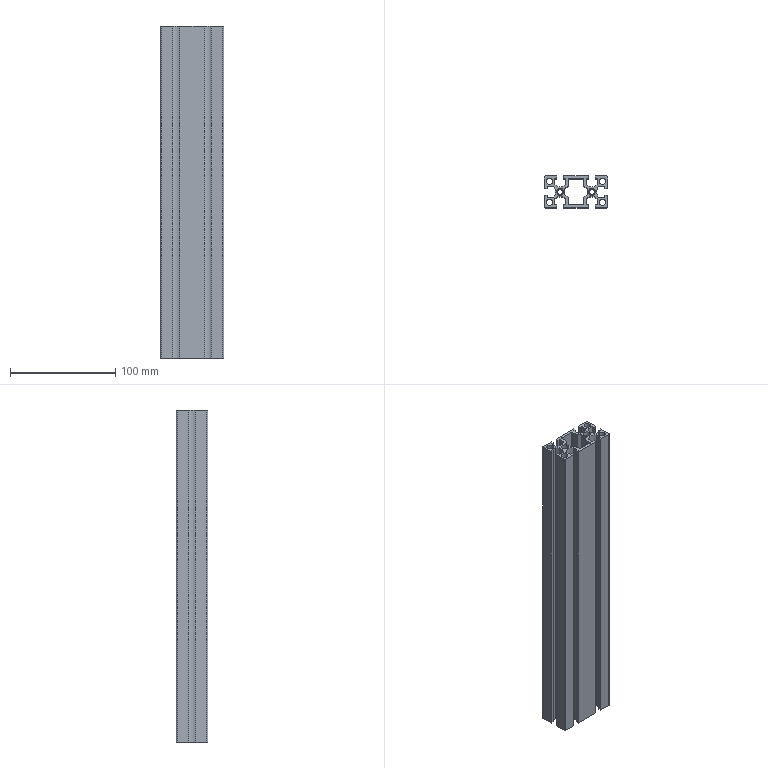Part | STEP file | 04-04 equal-height profile A | 1 solid | 103 faces | box 60 x 30 x 315 mm | volume 207544 mm3 | plane 60 | cylinder 35 | cone 8 | commonest cylinder face diameters 2 x8 6 x8 6.8 x8 15 x7 5 x4